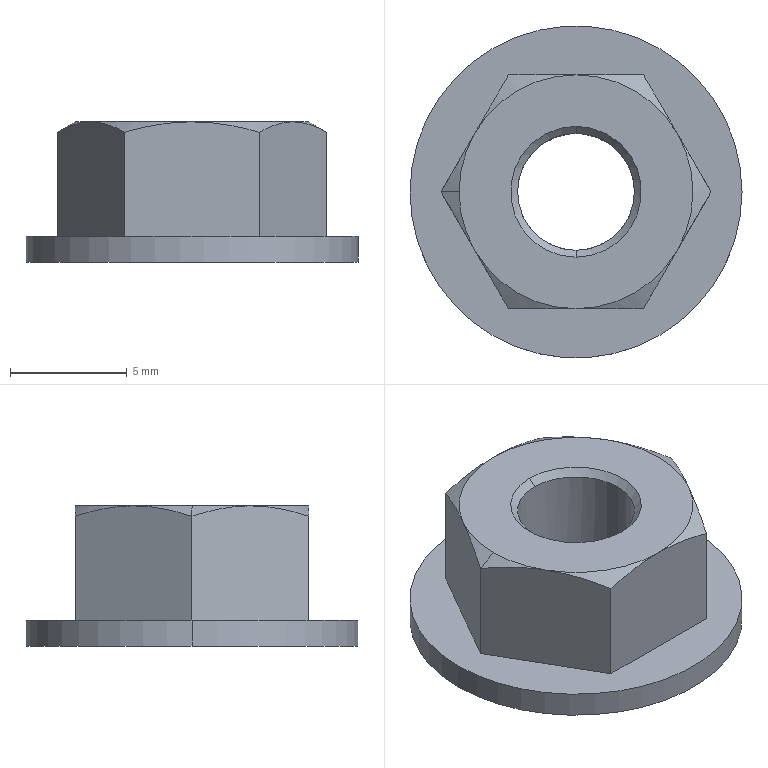Part | STEP file | LE-FL-M6_PN_0003 | 1 solid | 24 faces | box 14.2 x 14.2 x 6 mm | volume 478.178 mm3 | cone 11 | plane 9 | cylinder 4 | commonest cylinder face diameters 5 x2 14.2 x2
STEP:
#1=CARTESIAN_POINT('',(-7.1,0.,1.1));
#2=VERTEX_POINT('',#1);
#3=CARTESIAN_POINT('',(7.1,0.,1.1));
#4=VERTEX_POINT('',#3);
#5=CARTESIAN_POINT('',(0.,0.,1.1));
#6=DIRECTION('',(0.,0.,-1.));
#7=DIRECTION('',(-1.,0.,0.));
#8=AXIS2_PLACEMENT_3D('',#5,#6,#7);
#9=CIRCLE('',#8,7.1);
#10=EDGE_CURVE('',#2,#4,#9,.T.);
#11=ORIENTED_EDGE('',*,*,#10,.T.);
#12=CARTESIAN_POINT('',(7.1,0.,0.));
#13=VERTEX_POINT('',#12);
#14=CARTESIAN_POINT('',(7.1,0.,6.));
#15=DIRECTION('',(0.,0.,-1.));
#16=VECTOR('',#15,1000.);
#17=LINE('',#14,#16);
#18=EDGE_CURVE('',#4,#13,#17,.T.);
#19=ORIENTED_EDGE('',*,*,#18,.T.);
#20=CARTESIAN_POINT('',(-7.1,0.,0.));
#21=VERTEX_POINT('',#20);
#22=CARTESIAN_POINT('',(0.,0.,0.));
#23=DIRECTION('',(0.,0.,1.));
#24=DIRECTION('',(-1.,0.,0.));
#25=AXIS2_PLACEMENT_3D('',#22,#23,#24);
#26=CIRCLE('',#25,7.1);
#27=EDGE_CURVE('',#13,#21,#26,.T.);
#28=ORIENTED_EDGE('',*,*,#27,.T.);
#29=CARTESIAN_POINT('',(-7.1,0.,6.));
#30=DIRECTION('',(0.,0.,-1.));
#31=VECTOR('',#30,1000.);
#32=LINE('',#29,#31);
#33=EDGE_CURVE('',#2,#21,#32,.T.);
#34=ORIENTED_EDGE('',*,*,#33,.F.);
#35=EDGE_LOOP('',(#11,#19,#28,#34));
#36=FACE_OUTER_BOUND('',#35,.T.);
#37=CARTESIAN_POINT('',(0.,0.,6.));
#38=DIRECTION('',(0.,0.,-1.));
#39=DIRECTION('',(-1.,0.,0.));
#40=AXIS2_PLACEMENT_3D('',#37,#38,#39);
#41=CYLINDRICAL_SURFACE('',#40,7.1);
#42=ADVANCED_FACE('',(#36),#41,.T.);
#43=CARTESIAN_POINT('',(2.5,0.,0.3));
#44=VERTEX_POINT('',#43);
#45=CARTESIAN_POINT('',(-2.5,0.,0.3));
#46=VERTEX_POINT('',#45);
#47=CARTESIAN_POINT('',(0.,0.,0.3));
#48=DIRECTION('',(0.,0.,-1.));
#49=DIRECTION('',(-1.,0.,0.));
#50=AXIS2_PLACEMENT_3D('',#47,#48,#49);
#51=CIRCLE('',#50,2.5);
#52=EDGE_CURVE('',#44,#46,#51,.T.);
#53=ORIENTED_EDGE('',*,*,#52,.F.);
#54=CARTESIAN_POINT('',(2.8,0.,0.));
#55=VERTEX_POINT('',#54);
#56=CARTESIAN_POINT('',(2.8,0.,0.));
#57=DIRECTION('',(0.7071,0.,-0.7071));
#58=VECTOR('',#57,1000.);
#59=LINE('',#56,#58);
#60=EDGE_CURVE('',#44,#55,#59,.T.);
#61=ORIENTED_EDGE('',*,*,#60,.T.);
#62=CARTESIAN_POINT('',(-2.8,0.,0.));
#63=VERTEX_POINT('',#62);
#64=CARTESIAN_POINT('',(0.,0.,0.));
#65=DIRECTION('',(0.,0.,-1.));
#66=DIRECTION('',(-1.,0.,0.));
#67=AXIS2_PLACEMENT_3D('',#64,#65,#66);
#68=CIRCLE('',#67,2.8);
#69=EDGE_CURVE('',#55,#63,#68,.T.);
#70=ORIENTED_EDGE('',*,*,#69,.T.);
#71=CARTESIAN_POINT('',(-2.8,0.,0.));
#72=DIRECTION('',(-0.7071,0.,-0.7071));
#73=VECTOR('',#72,1000.);
#74=LINE('',#71,#73);
#75=EDGE_CURVE('',#46,#63,#74,.T.);
#76=ORIENTED_EDGE('',*,*,#75,.F.);
#77=EDGE_LOOP('',(#53,#61,#70,#76));
#78=FACE_OUTER_BOUND('',#77,.T.);
#79=CARTESIAN_POINT('',(0.,0.,0.));
#80=DIRECTION('',(0.,0.,-1.));
#81=DIRECTION('',(-1.,0.,0.));
#82=AXIS2_PLACEMENT_3D('',#79,#80,#81);
#83=CONICAL_SURFACE('',#82,2.8,0.7854);
#84=ADVANCED_FACE('',(#78),#83,.F.);
#85=ORIENTED_EDGE('',*,*,#52,.T.);
#86=CARTESIAN_POINT('',(-2.5,0.,5.7));
#87=VERTEX_POINT('',#86);
#88=CARTESIAN_POINT('',(-2.5,0.,6.));
#89=DIRECTION('',(0.,0.,1.));
#90=VECTOR('',#89,1000.);
#91=LINE('',#88,#90);
#92=EDGE_CURVE('',#46,#87,#91,.T.);
#93=ORIENTED_EDGE('',*,*,#92,.T.);
#94=CARTESIAN_POINT('',(0.,-2.5,5.7));
#95=VERTEX_POINT('',#94);
#96=CARTESIAN_POINT('',(0.,0.,5.7));
#97=DIRECTION('',(0.,0.,-1.));
#98=DIRECTION('',(1.,0.,0.));
#99=AXIS2_PLACEMENT_3D('',#96,#97,#98);
#100=CIRCLE('',#99,2.5);
#101=EDGE_CURVE('',#95,#87,#100,.T.);
#102=ORIENTED_EDGE('',*,*,#101,.F.);
#103=CARTESIAN_POINT('',(2.5,0.,5.7));
#104=VERTEX_POINT('',#103);
#105=CARTESIAN_POINT('',(0.,0.,5.7));
#106=DIRECTION('',(0.,0.,-1.));
#107=DIRECTION('',(1.,0.,0.));
#108=AXIS2_PLACEMENT_3D('',#105,#106,#107);
#109=CIRCLE('',#108,2.5);
#110=EDGE_CURVE('',#104,#95,#109,.T.);
#111=ORIENTED_EDGE('',*,*,#110,.F.);
#112=CARTESIAN_POINT('',(2.5,0.,6.));
#113=DIRECTION('',(0.,0.,1.));
#114=VECTOR('',#113,1000.);
#115=LINE('',#112,#114);
#116=EDGE_CURVE('',#44,#104,#115,.T.);
#117=ORIENTED_EDGE('',*,*,#116,.F.);
#118=EDGE_LOOP('',(#85,#93,#102,#111,#117));
#119=FACE_OUTER_BOUND('',#118,.T.);
#120=CARTESIAN_POINT('',(0.,0.,6.));
#121=DIRECTION('',(0.,0.,1.));
#122=DIRECTION('',(1.,0.,0.));
#123=AXIS2_PLACEMENT_3D('',#120,#121,#122);
#124=CYLINDRICAL_SURFACE('',#123,2.5);
#125=ADVANCED_FACE('',(#119),#124,.F.);
#126=ORIENTED_EDGE('',*,*,#101,.T.);
#127=CARTESIAN_POINT('',(0.,2.5,5.7));
#128=VERTEX_POINT('',#127);
#129=CARTESIAN_POINT('',(0.,0.,5.7));
#130=DIRECTION('',(0.,0.,-1.));
#131=DIRECTION('',(1.,0.,0.));
#132=AXIS2_PLACEMENT_3D('',#129,#130,#131);
#133=CIRCLE('',#132,2.5);
#134=EDGE_CURVE('',#87,#128,#133,.T.);
#135=ORIENTED_EDGE('',*,*,#134,.T.);
#136=CARTESIAN_POINT('',(0.,2.8,6.));
#137=VERTEX_POINT('',#136);
#138=CARTESIAN_POINT('',(0.,2.8,6.));
#139=DIRECTION('',(0.,0.7071,0.7071));
#140=VECTOR('',#139,1000.);
#141=LINE('',#138,#140);
#142=EDGE_CURVE('',#128,#137,#141,.T.);
#143=ORIENTED_EDGE('',*,*,#142,.T.);
#144=CARTESIAN_POINT('',(0.,-2.8,6.));
#145=VERTEX_POINT('',#144);
#146=CARTESIAN_POINT('',(0.,0.,6.));
#147=DIRECTION('',(0.,0.,-1.));
#148=DIRECTION('',(0.,-1.,0.));
#149=AXIS2_PLACEMENT_3D('',#146,#147,#148);
#150=CIRCLE('',#149,2.8);
#151=EDGE_CURVE('',#145,#137,#150,.T.);
#152=ORIENTED_EDGE('',*,*,#151,.F.);
#153=CARTESIAN_POINT('',(0.,-2.8,6.));
#154=DIRECTION('',(0.,-0.7071,0.7071));
#155=VECTOR('',#154,1000.);
#156=LINE('',#153,#155);
#157=EDGE_CURVE('',#95,#145,#156,.T.);
#158=ORIENTED_EDGE('',*,*,#157,.F.);
#159=EDGE_LOOP('',(#126,#135,#143,#152,#158));
#160=FACE_OUTER_BOUND('',#159,.T.);
#161=CARTESIAN_POINT('',(0.,0.,6.));
#162=DIRECTION('',(0.,0.,1.));
#163=DIRECTION('',(0.,-1.,0.));
#164=AXIS2_PLACEMENT_3D('',#161,#162,#163);
#165=CONICAL_SURFACE('',#164,2.8,0.7854);
#166=ADVANCED_FACE('',(#160),#165,.F.);
#167=CARTESIAN_POINT('',(-4.33,-2.5,6.));
#168=VERTEX_POINT('',#167);
#169=CARTESIAN_POINT('',(-5.,0.,6.));
#170=VERTEX_POINT('',#169);
#171=CARTESIAN_POINT('',(0.,0.,6.));
#172=DIRECTION('',(0.,0.,-1.));
#173=DIRECTION('',(-1.,0.,0.));
#174=AXIS2_PLACEMENT_3D('',#171,#172,#173);
#175=CIRCLE('',#174,5.);
#176=EDGE_CURVE('',#168,#170,#175,.T.);
#177=ORIENTED_EDGE('',*,*,#176,.T.);
#178=CARTESIAN_POINT('',(-5.774,0.,5.553));
#179=VERTEX_POINT('',#178);
#180=CARTESIAN_POINT('',(-5.778,0.,5.551));
#181=DIRECTION('',(-0.866,0.,-0.5));
#182=VECTOR('',#181,1000.);
#183=LINE('',#180,#182);
#184=EDGE_CURVE('',#170,#179,#183,.T.);
#185=ORIENTED_EDGE('',*,*,#184,.T.);
#186=CARTESIAN_POINT('',(-4.33,-2.5,6.));
#187=CARTESIAN_POINT('',(-4.823,-1.647,6.));
#188=CARTESIAN_POINT('',(-5.302,-0.8168,5.826));
#189=CARTESIAN_POINT('',(-5.774,0.,5.553));
#190=B_SPLINE_CURVE_WITH_KNOTS('',3,(#186,#187,#188,#189),.UNSPECIFIED.,.F.,.F.,(4,4),(0.,0.002921),.UNSPECIFIED.);
#191=EDGE_CURVE('',#168,#179,#190,.T.);
#192=ORIENTED_EDGE('',*,*,#191,.F.);
#193=EDGE_LOOP('',(#177,#185,#192));
#194=FACE_OUTER_BOUND('',#193,.T.);
#195=CARTESIAN_POINT('',(0.,0.,5.551));
#196=DIRECTION('',(0.,0.,-1.));
#197=DIRECTION('',(-1.,0.,0.));
#198=AXIS2_PLACEMENT_3D('',#195,#196,#197);
#199=CONICAL_SURFACE('',#198,5.778,1.047);
#200=ADVANCED_FACE('',(#194),#199,.T.);
#201=CARTESIAN_POINT('',(0.,0.,0.));
#202=DIRECTION('',(0.,0.,1.));
#203=DIRECTION('',(-1.,0.,0.));
#204=AXIS2_PLACEMENT_3D('',#201,#202,#203);
#205=CIRCLE('',#204,7.1);
#206=EDGE_CURVE('',#21,#13,#205,.T.);
#207=ORIENTED_EDGE('',*,*,#206,.F.);
#208=ORIENTED_EDGE('',*,*,#27,.F.);
#209=EDGE_LOOP('',(#207,#208));
#210=FACE_OUTER_BOUND('',#209,.T.);
#211=CARTESIAN_POINT('',(0.,0.,0.));
#212=DIRECTION('',(0.,0.,-1.));
#213=DIRECTION('',(-1.,0.,0.));
#214=AXIS2_PLACEMENT_3D('',#211,#212,#213);
#215=CIRCLE('',#214,2.8);
#216=EDGE_CURVE('',#63,#55,#215,.T.);
#217=ORIENTED_EDGE('',*,*,#216,.F.);
#218=ORIENTED_EDGE('',*,*,#69,.F.);
#219=EDGE_LOOP('',(#217,#218));
#220=FACE_BOUND('',#219,.T.);
#221=CARTESIAN_POINT('',(0.,0.,0.));
#222=DIRECTION('',(0.,0.,1.));
#223=DIRECTION('',(1.,0.,0.));
#224=AXIS2_PLACEMENT_3D('',#221,#222,#223);
#225=PLANE('',#224);
#226=ADVANCED_FACE('',(#210,#220),#225,.F.);
#227=ORIENTED_EDGE('',*,*,#18,.F.);
#228=CARTESIAN_POINT('',(0.,0.,1.1));
#229=DIRECTION('',(0.,0.,-1.));
#230=DIRECTION('',(-1.,0.,0.));
#231=AXIS2_PLACEMENT_3D('',#228,#229,#230);
#232=CIRCLE('',#231,7.1);
#233=EDGE_CURVE('',#4,#2,#232,.T.);
#234=ORIENTED_EDGE('',*,*,#233,.T.);
#235=ORIENTED_EDGE('',*,*,#33,.T.);
#236=ORIENTED_EDGE('',*,*,#206,.T.);
#237=EDGE_LOOP('',(#227,#234,#235,#236));
#238=FACE_OUTER_BOUND('',#237,.T.);
#239=CARTESIAN_POINT('',(0.,0.,6.));
#240=DIRECTION('',(0.,0.,-1.));
#241=DIRECTION('',(-1.,0.,0.));
#242=AXIS2_PLACEMENT_3D('',#239,#240,#241);
#243=CYLINDRICAL_SURFACE('',#242,7.1);
#244=ADVANCED_FACE('',(#238),#243,.T.);
#245=ORIENTED_EDGE('',*,*,#60,.F.);
#246=CARTESIAN_POINT('',(0.,0.,0.3));
#247=DIRECTION('',(0.,0.,-1.));
#248=DIRECTION('',(-1.,0.,0.));
#249=AXIS2_PLACEMENT_3D('',#246,#247,#248);
#250=CIRCLE('',#249,2.5);
#251=EDGE_CURVE('',#46,#44,#250,.T.);
#252=ORIENTED_EDGE('',*,*,#251,.F.);
#253=ORIENTED_EDGE('',*,*,#75,.T.);
#254=ORIENTED_EDGE('',*,*,#216,.T.);
#255=EDGE_LOOP('',(#245,#252,#253,#254));
#256=FACE_OUTER_BOUND('',#255,.T.);
#257=CARTESIAN_POINT('',(0.,0.,0.));
#258=DIRECTION('',(0.,0.,-1.));
#259=DIRECTION('',(-1.,0.,0.));
#260=AXIS2_PLACEMENT_3D('',#257,#258,#259);
#261=CONICAL_SURFACE('',#260,2.8,0.7854);
#262=ADVANCED_FACE('',(#256),#261,.F.);
#263=ORIENTED_EDGE('',*,*,#10,.F.);
#264=ORIENTED_EDGE('',*,*,#233,.F.);
#265=EDGE_LOOP('',(#263,#264));
#266=FACE_OUTER_BOUND('',#265,.T.);
#267=CARTESIAN_POINT('',(-2.887,5.,1.1));
#268=VERTEX_POINT('',#267);
#269=CARTESIAN_POINT('',(2.887,5.,1.1));
#270=VERTEX_POINT('',#269);
#271=CARTESIAN_POINT('',(0.,5.,1.1));
#272=DIRECTION('',(1.,0.,0.));
#273=VECTOR('',#272,1000.);
#274=LINE('',#271,#273);
#275=EDGE_CURVE('',#268,#270,#274,.T.);
#276=ORIENTED_EDGE('',*,*,#275,.T.);
#277=CARTESIAN_POINT('',(5.774,0.,1.1));
#278=VERTEX_POINT('',#277);
#279=CARTESIAN_POINT('',(2.887,5.,1.1));
#280=DIRECTION('',(0.5,-0.866,0.));
#281=VECTOR('',#280,1000.);
#282=LINE('',#279,#281);
#283=EDGE_CURVE('',#270,#278,#282,.T.);
#284=ORIENTED_EDGE('',*,*,#283,.T.);
#285=CARTESIAN_POINT('',(2.887,-5.,1.1));
#286=VERTEX_POINT('',#285);
#287=CARTESIAN_POINT('',(5.774,0.,1.1));
#288=DIRECTION('',(-0.5,-0.866,0.));
#289=VECTOR('',#288,1000.);
#290=LINE('',#287,#289);
#291=EDGE_CURVE('',#278,#286,#290,.T.);
#292=ORIENTED_EDGE('',*,*,#291,.T.);
#293=CARTESIAN_POINT('',(-2.887,-5.,1.1));
#294=VERTEX_POINT('',#293);
#295=CARTESIAN_POINT('',(0.,-5.,1.1));
#296=DIRECTION('',(-1.,0.,0.));
#297=VECTOR('',#296,1000.);
#298=LINE('',#295,#297);
#299=EDGE_CURVE('',#286,#294,#298,.T.);
#300=ORIENTED_EDGE('',*,*,#299,.T.);
#301=CARTESIAN_POINT('',(-5.774,0.,1.1));
#302=VERTEX_POINT('',#301);
#303=CARTESIAN_POINT('',(-2.887,-5.,1.1));
#304=DIRECTION('',(-0.5,0.866,0.));
#305=VECTOR('',#304,1000.);
#306=LINE('',#303,#305);
#307=EDGE_CURVE('',#294,#302,#306,.T.);
#308=ORIENTED_EDGE('',*,*,#307,.T.);
#309=CARTESIAN_POINT('',(-5.774,0.,1.1));
#310=DIRECTION('',(0.5,0.866,0.));
#311=VECTOR('',#310,1000.);
#312=LINE('',#309,#311);
#313=EDGE_CURVE('',#302,#268,#312,.T.);
#314=ORIENTED_EDGE('',*,*,#313,.T.);
#315=EDGE_LOOP('',(#276,#284,#292,#300,#308,#314));
#316=FACE_BOUND('',#315,.T.);
#317=CARTESIAN_POINT('',(0.,0.,1.1));
#318=DIRECTION('',(0.,0.,1.));
#319=DIRECTION('',(1.,0.,0.));
#320=AXIS2_PLACEMENT_3D('',#317,#318,#319);
#321=PLANE('',#320);
#322=ADVANCED_FACE('',(#266,#316),#321,.T.);
#323=ORIENTED_EDGE('',*,*,#92,.F.);
#324=ORIENTED_EDGE('',*,*,#251,.T.);
#325=ORIENTED_EDGE('',*,*,#116,.T.);
#326=CARTESIAN_POINT('',(0.,0.,5.7));
#327=DIRECTION('',(0.,0.,-1.));
#328=DIRECTION('',(1.,0.,0.));
#329=AXIS2_PLACEMENT_3D('',#326,#327,#328);
#330=CIRCLE('',#329,2.5);
#331=EDGE_CURVE('',#128,#104,#330,.T.);
#332=ORIENTED_EDGE('',*,*,#331,.F.);
#333=ORIENTED_EDGE('',*,*,#134,.F.);
#334=EDGE_LOOP('',(#323,#324,#325,#332,#333));
#335=FACE_OUTER_BOUND('',#334,.T.);
#336=CARTESIAN_POINT('',(0.,0.,6.));
#337=DIRECTION('',(0.,0.,1.));
#338=DIRECTION('',(1.,0.,0.));
#339=AXIS2_PLACEMENT_3D('',#336,#337,#338);
#340=CYLINDRICAL_SURFACE('',#339,2.5);
#341=ADVANCED_FACE('',(#335),#340,.F.);
#342=CARTESIAN_POINT('',(2.887,5.,5.553));
#343=VERTEX_POINT('',#342);
#344=CARTESIAN_POINT('',(4.33,2.5,6.));
#345=VERTEX_POINT('',#344);
#346=CARTESIAN_POINT('',(2.887,5.,5.553));
#347=CARTESIAN_POINT('',(3.358,4.183,5.826));
#348=CARTESIAN_POINT('',(3.837,3.353,6.));
#349=CARTESIAN_POINT('',(4.33,2.5,6.));
#350=B_SPLINE_CURVE_WITH_KNOTS('',3,(#346,#347,#348,#349),.UNSPECIFIED.,.F.,.F.,(4,4),(0.,0.002921),.UNSPECIFIED.);
#351=EDGE_CURVE('',#343,#345,#350,.T.);
#352=ORIENTED_EDGE('',*,*,#351,.T.);
#353=CARTESIAN_POINT('',(5.774,0.,5.553));
#354=VERTEX_POINT('',#353);
#355=CARTESIAN_POINT('',(4.33,2.5,6.));
#356=CARTESIAN_POINT('',(4.823,1.647,6.));
#357=CARTESIAN_POINT('',(5.302,0.8168,5.826));
#358=CARTESIAN_POINT('',(5.774,0.,5.553));
#359=B_SPLINE_CURVE_WITH_KNOTS('',3,(#355,#356,#357,#358),.UNSPECIFIED.,.F.,.F.,(4,4),(0.,0.002921),.UNSPECIFIED.);
#360=EDGE_CURVE('',#345,#354,#359,.T.);
#361=ORIENTED_EDGE('',*,*,#360,.T.);
#362=CARTESIAN_POINT('',(5.774,0.,1.1));
#363=DIRECTION('',(0.,0.,-1.));
#364=VECTOR('',#363,1000.);
#365=LINE('',#362,#364);
#366=EDGE_CURVE('',#354,#278,#365,.T.);
#367=ORIENTED_EDGE('',*,*,#366,.T.);
#368=ORIENTED_EDGE('',*,*,#283,.F.);
#369=CARTESIAN_POINT('',(2.887,5.,1.1));
#370=DIRECTION('',(0.,0.,1.));
#371=VECTOR('',#370,1000.);
#372=LINE('',#369,#371);
#373=EDGE_CURVE('',#270,#343,#372,.T.);
#374=ORIENTED_EDGE('',*,*,#373,.T.);
#375=EDGE_LOOP('',(#352,#361,#367,#368,#374));
#376=FACE_OUTER_BOUND('',#375,.T.);
#377=CARTESIAN_POINT('',(5.774,0.,1.1));
#378=DIRECTION('',(0.866,0.5,0.));
#379=DIRECTION('',(-0.5,0.866,0.));
#380=AXIS2_PLACEMENT_3D('',#377,#378,#379);
#381=PLANE('',#380);
#382=ADVANCED_FACE('',(#376),#381,.T.);
#383=CARTESIAN_POINT('',(-2.887,5.,5.553));
#384=VERTEX_POINT('',#383);
#385=CARTESIAN_POINT('',(0.,5.,6.));
#386=VERTEX_POINT('',#385);
#387=CARTESIAN_POINT('',(-2.887,5.,5.553));
#388=CARTESIAN_POINT('',(-1.944,5.,5.826));
#389=CARTESIAN_POINT('',(-0.9853,5.,6.));
#390=CARTESIAN_POINT('',(0.,5.,6.));
#391=B_SPLINE_CURVE_WITH_KNOTS('',3,(#387,#388,#389,#390),.UNSPECIFIED.,.F.,.F.,(4,4),(0.,0.002921),.UNSPECIFIED.);
#392=EDGE_CURVE('',#384,#386,#391,.T.);
#393=ORIENTED_EDGE('',*,*,#392,.T.);
#394=CARTESIAN_POINT('',(0.,5.,6.));
#395=CARTESIAN_POINT('',(0.9853,5.,6.));
#396=CARTESIAN_POINT('',(1.944,5.,5.826));
#397=CARTESIAN_POINT('',(2.887,5.,5.553));
#398=B_SPLINE_CURVE_WITH_KNOTS('',3,(#394,#395,#396,#397),.UNSPECIFIED.,.F.,.F.,(4,4),(0.,0.002921),.UNSPECIFIED.);
#399=EDGE_CURVE('',#386,#343,#398,.T.);
#400=ORIENTED_EDGE('',*,*,#399,.T.);
#401=ORIENTED_EDGE('',*,*,#373,.F.);
#402=ORIENTED_EDGE('',*,*,#275,.F.);
#403=CARTESIAN_POINT('',(-2.887,5.,1.1));
#404=DIRECTION('',(0.,0.,1.));
#405=VECTOR('',#404,1000.);
#406=LINE('',#403,#405);
#407=EDGE_CURVE('',#268,#384,#406,.T.);
#408=ORIENTED_EDGE('',*,*,#407,.T.);
#409=EDGE_LOOP('',(#393,#400,#401,#402,#408));
#410=FACE_OUTER_BOUND('',#409,.T.);
#411=CARTESIAN_POINT('',(2.887,5.,1.1));
#412=DIRECTION('',(0.,1.,0.));
#413=DIRECTION('',(0.,0.,1.));
#414=AXIS2_PLACEMENT_3D('',#411,#412,#413);
#415=PLANE('',#414);
#416=ADVANCED_FACE('',(#410),#415,.T.);
#417=CARTESIAN_POINT('',(-4.33,2.5,6.));
#418=VERTEX_POINT('',#417);
#419=CARTESIAN_POINT('',(-5.774,0.,5.553));
#420=CARTESIAN_POINT('',(-5.302,0.8168,5.826));
#421=CARTESIAN_POINT('',(-4.823,1.647,6.));
#422=CARTESIAN_POINT('',(-4.33,2.5,6.));
#423=B_SPLINE_CURVE_WITH_KNOTS('',3,(#419,#420,#421,#422),.UNSPECIFIED.,.F.,.F.,(4,4),(0.,0.002921),.UNSPECIFIED.);
#424=EDGE_CURVE('',#179,#418,#423,.T.);
#425=ORIENTED_EDGE('',*,*,#424,.T.);
#426=CARTESIAN_POINT('',(-4.33,2.5,6.));
#427=CARTESIAN_POINT('',(-3.837,3.353,6.));
#428=CARTESIAN_POINT('',(-3.358,4.183,5.826));
#429=CARTESIAN_POINT('',(-2.887,5.,5.553));
#430=B_SPLINE_CURVE_WITH_KNOTS('',3,(#426,#427,#428,#429),.UNSPECIFIED.,.F.,.F.,(4,4),(0.,0.002921),.UNSPECIFIED.);
#431=EDGE_CURVE('',#418,#384,#430,.T.);
#432=ORIENTED_EDGE('',*,*,#431,.T.);
#433=ORIENTED_EDGE('',*,*,#407,.F.);
#434=ORIENTED_EDGE('',*,*,#313,.F.);
#435=CARTESIAN_POINT('',(-5.774,0.,1.1));
#436=DIRECTION('',(0.,0.,1.));
#437=VECTOR('',#436,1000.);
#438=LINE('',#435,#437);
#439=EDGE_CURVE('',#302,#179,#438,.T.);
#440=ORIENTED_EDGE('',*,*,#439,.T.);
#441=EDGE_LOOP('',(#425,#432,#433,#434,#440));
#442=FACE_OUTER_BOUND('',#441,.T.);
#443=CARTESIAN_POINT('',(-2.887,5.,1.1));
#444=DIRECTION('',(-0.866,0.5,0.));
#445=DIRECTION('',(-0.5,-0.866,0.));
#446=AXIS2_PLACEMENT_3D('',#443,#444,#445);
#447=PLANE('',#446);
#448=ADVANCED_FACE('',(#442),#447,.T.);
#449=CARTESIAN_POINT('',(-2.887,-5.,5.553));
#450=VERTEX_POINT('',#449);
#451=CARTESIAN_POINT('',(-2.887,-5.,5.553));
#452=CARTESIAN_POINT('',(-3.358,-4.183,5.826));
#453=CARTESIAN_POINT('',(-3.837,-3.353,6.));
#454=CARTESIAN_POINT('',(-4.33,-2.5,6.));
#455=B_SPLINE_CURVE_WITH_KNOTS('',3,(#451,#452,#453,#454),.UNSPECIFIED.,.F.,.F.,(4,4),(0.,0.002921),.UNSPECIFIED.);
#456=EDGE_CURVE('',#450,#168,#455,.T.);
#457=ORIENTED_EDGE('',*,*,#456,.T.);
#458=ORIENTED_EDGE('',*,*,#191,.T.);
#459=ORIENTED_EDGE('',*,*,#439,.F.);
#460=ORIENTED_EDGE('',*,*,#307,.F.);
#461=CARTESIAN_POINT('',(-2.887,-5.,1.1));
#462=DIRECTION('',(0.,0.,1.));
#463=VECTOR('',#462,1000.);
#464=LINE('',#461,#463);
#465=EDGE_CURVE('',#294,#450,#464,.T.);
#466=ORIENTED_EDGE('',*,*,#465,.T.);
#467=EDGE_LOOP('',(#457,#458,#459,#460,#466));
#468=FACE_OUTER_BOUND('',#467,.T.);
#469=CARTESIAN_POINT('',(-5.774,0.,1.1));
#470=DIRECTION('',(-0.866,-0.5,0.));
#471=DIRECTION('',(0.5,-0.866,0.));
#472=AXIS2_PLACEMENT_3D('',#469,#470,#471);
#473=PLANE('',#472);
#474=ADVANCED_FACE('',(#468),#473,.T.);
#475=CARTESIAN_POINT('',(2.887,-5.,5.553));
#476=VERTEX_POINT('',#475);
#477=CARTESIAN_POINT('',(0.,-5.,6.));
#478=VERTEX_POINT('',#477);
#479=CARTESIAN_POINT('',(2.887,-5.,5.553));
#480=CARTESIAN_POINT('',(1.944,-5.,5.826));
#481=CARTESIAN_POINT('',(0.9853,-5.,6.));
#482=CARTESIAN_POINT('',(0.,-5.,6.));
#483=B_SPLINE_CURVE_WITH_KNOTS('',3,(#479,#480,#481,#482),.UNSPECIFIED.,.F.,.F.,(4,4),(0.,0.002921),.UNSPECIFIED.);
#484=EDGE_CURVE('',#476,#478,#483,.T.);
#485=ORIENTED_EDGE('',*,*,#484,.T.);
#486=CARTESIAN_POINT('',(0.,-5.,6.));
#487=CARTESIAN_POINT('',(-0.9853,-5.,6.));
#488=CARTESIAN_POINT('',(-1.944,-5.,5.826));
#489=CARTESIAN_POINT('',(-2.887,-5.,5.553));
#490=B_SPLINE_CURVE_WITH_KNOTS('',3,(#486,#487,#488,#489),.UNSPECIFIED.,.F.,.F.,(4,4),(0.,0.002921),.UNSPECIFIED.);
#491=EDGE_CURVE('',#478,#450,#490,.T.);
#492=ORIENTED_EDGE('',*,*,#491,.T.);
#493=ORIENTED_EDGE('',*,*,#465,.F.);
#494=ORIENTED_EDGE('',*,*,#299,.F.);
#495=CARTESIAN_POINT('',(2.887,-5.,1.1));
#496=DIRECTION('',(0.,0.,1.));
#497=VECTOR('',#496,1000.);
#498=LINE('',#495,#497);
#499=EDGE_CURVE('',#286,#476,#498,.T.);
#500=ORIENTED_EDGE('',*,*,#499,.T.);
#501=EDGE_LOOP('',(#485,#492,#493,#494,#500));
#502=FACE_OUTER_BOUND('',#501,.T.);
#503=CARTESIAN_POINT('',(-2.887,-5.,1.1));
#504=DIRECTION('',(0.,-1.,0.));
#505=DIRECTION('',(0.,0.,-1.));
#506=AXIS2_PLACEMENT_3D('',#503,#504,#505);
#507=PLANE('',#506);
#508=ADVANCED_FACE('',(#502),#507,.T.);
#509=CARTESIAN_POINT('',(4.33,-2.5,6.));
#510=VERTEX_POINT('',#509);
#511=CARTESIAN_POINT('',(5.774,0.,5.553));
#512=CARTESIAN_POINT('',(5.302,-0.8168,5.826));
#513=CARTESIAN_POINT('',(4.823,-1.647,6.));
#514=CARTESIAN_POINT('',(4.33,-2.5,6.));
#515=B_SPLINE_CURVE_WITH_KNOTS('',3,(#511,#512,#513,#514),.UNSPECIFIED.,.F.,.F.,(4,4),(0.,0.002921),.UNSPECIFIED.);
#516=EDGE_CURVE('',#354,#510,#515,.T.);
#517=ORIENTED_EDGE('',*,*,#516,.T.);
#518=CARTESIAN_POINT('',(4.33,-2.5,6.));
#519=CARTESIAN_POINT('',(3.837,-3.353,6.));
#520=CARTESIAN_POINT('',(3.358,-4.183,5.826));
#521=CARTESIAN_POINT('',(2.887,-5.,5.553));
#522=B_SPLINE_CURVE_WITH_KNOTS('',3,(#518,#519,#520,#521),.UNSPECIFIED.,.F.,.F.,(4,4),(0.,0.002921),.UNSPECIFIED.);
#523=EDGE_CURVE('',#510,#476,#522,.T.);
#524=ORIENTED_EDGE('',*,*,#523,.T.);
#525=ORIENTED_EDGE('',*,*,#499,.F.);
#526=ORIENTED_EDGE('',*,*,#291,.F.);
#527=ORIENTED_EDGE('',*,*,#366,.F.);
#528=EDGE_LOOP('',(#517,#524,#525,#526,#527));
#529=FACE_OUTER_BOUND('',#528,.T.);
#530=CARTESIAN_POINT('',(2.887,-5.,1.1));
#531=DIRECTION('',(0.866,-0.5,0.));
#532=DIRECTION('',(0.5,0.866,0.));
#533=AXIS2_PLACEMENT_3D('',#530,#531,#532);
#534=PLANE('',#533);
#535=ADVANCED_FACE('',(#529),#534,.T.);
#536=ORIENTED_EDGE('',*,*,#142,.F.);
#537=ORIENTED_EDGE('',*,*,#331,.T.);
#538=ORIENTED_EDGE('',*,*,#110,.T.);
#539=ORIENTED_EDGE('',*,*,#157,.T.);
#540=CARTESIAN_POINT('',(0.,0.,6.));
#541=DIRECTION('',(0.,0.,-1.));
#542=DIRECTION('',(0.,-1.,0.));
#543=AXIS2_PLACEMENT_3D('',#540,#541,#542);
#544=CIRCLE('',#543,2.8);
#545=EDGE_CURVE('',#137,#145,#544,.T.);
#546=ORIENTED_EDGE('',*,*,#545,.F.);
#547=EDGE_LOOP('',(#536,#537,#538,#539,#546));
#548=FACE_OUTER_BOUND('',#547,.T.);
#549=CARTESIAN_POINT('',(0.,0.,6.));
#550=DIRECTION('',(0.,0.,1.));
#551=DIRECTION('',(0.,-1.,0.));
#552=AXIS2_PLACEMENT_3D('',#549,#550,#551);
#553=CONICAL_SURFACE('',#552,2.8,0.7854);
#554=ADVANCED_FACE('',(#548),#553,.F.);
#555=ORIENTED_EDGE('',*,*,#516,.F.);
#556=ORIENTED_EDGE('',*,*,#360,.F.);
#557=CARTESIAN_POINT('',(0.,0.,6.));
#558=DIRECTION('',(0.,0.,-1.));
#559=DIRECTION('',(-1.,0.,0.));
#560=AXIS2_PLACEMENT_3D('',#557,#558,#559);
#561=CIRCLE('',#560,5.);
#562=EDGE_CURVE('',#345,#510,#561,.T.);
#563=ORIENTED_EDGE('',*,*,#562,.T.);
#564=EDGE_LOOP('',(#555,#556,#563));
#565=FACE_OUTER_BOUND('',#564,.T.);
#566=CARTESIAN_POINT('',(0.,0.,5.551));
#567=DIRECTION('',(0.,0.,-1.));
#568=DIRECTION('',(-1.,0.,0.));
#569=AXIS2_PLACEMENT_3D('',#566,#567,#568);
#570=CONICAL_SURFACE('',#569,5.778,1.047);
#571=ADVANCED_FACE('',(#565),#570,.T.);
#572=ORIENTED_EDGE('',*,*,#351,.F.);
#573=ORIENTED_EDGE('',*,*,#399,.F.);
#574=CARTESIAN_POINT('',(0.,0.,6.));
#575=DIRECTION('',(0.,0.,-1.));
#576=DIRECTION('',(-1.,0.,0.));
#577=AXIS2_PLACEMENT_3D('',#574,#575,#576);
#578=CIRCLE('',#577,5.);
#579=EDGE_CURVE('',#386,#345,#578,.T.);
#580=ORIENTED_EDGE('',*,*,#579,.T.);
#581=EDGE_LOOP('',(#572,#573,#580));
#582=FACE_OUTER_BOUND('',#581,.T.);
#583=CARTESIAN_POINT('',(0.,0.,5.551));
#584=DIRECTION('',(0.,0.,-1.));
#585=DIRECTION('',(-1.,0.,0.));
#586=AXIS2_PLACEMENT_3D('',#583,#584,#585);
#587=CONICAL_SURFACE('',#586,5.778,1.047);
#588=ADVANCED_FACE('',(#582),#587,.T.);
#589=ORIENTED_EDGE('',*,*,#431,.F.);
#590=CARTESIAN_POINT('',(0.,0.,6.));
#591=DIRECTION('',(0.,0.,-1.));
#592=DIRECTION('',(-1.,0.,0.));
#593=AXIS2_PLACEMENT_3D('',#590,#591,#592);
#594=CIRCLE('',#593,5.);
#595=EDGE_CURVE('',#418,#386,#594,.T.);
#596=ORIENTED_EDGE('',*,*,#595,.T.);
#597=ORIENTED_EDGE('',*,*,#392,.F.);
#598=EDGE_LOOP('',(#589,#596,#597));
#599=FACE_OUTER_BOUND('',#598,.T.);
#600=CARTESIAN_POINT('',(0.,0.,5.551));
#601=DIRECTION('',(0.,0.,-1.));
#602=DIRECTION('',(-1.,0.,0.));
#603=AXIS2_PLACEMENT_3D('',#600,#601,#602);
#604=CONICAL_SURFACE('',#603,5.778,1.047);
#605=ADVANCED_FACE('',(#599),#604,.T.);
#606=ORIENTED_EDGE('',*,*,#184,.F.);
#607=CARTESIAN_POINT('',(0.,0.,6.));
#608=DIRECTION('',(0.,0.,-1.));
#609=DIRECTION('',(-1.,0.,0.));
#610=AXIS2_PLACEMENT_3D('',#607,#608,#609);
#611=CIRCLE('',#610,5.);
#612=EDGE_CURVE('',#170,#418,#611,.T.);
#613=ORIENTED_EDGE('',*,*,#612,.T.);
#614=ORIENTED_EDGE('',*,*,#424,.F.);
#615=EDGE_LOOP('',(#606,#613,#614));
#616=FACE_OUTER_BOUND('',#615,.T.);
#617=CARTESIAN_POINT('',(0.,0.,5.551));
#618=DIRECTION('',(0.,0.,-1.));
#619=DIRECTION('',(-1.,0.,0.));
#620=AXIS2_PLACEMENT_3D('',#617,#618,#619);
#621=CONICAL_SURFACE('',#620,5.778,1.047);
#622=ADVANCED_FACE('',(#616),#621,.T.);
#623=ORIENTED_EDGE('',*,*,#491,.F.);
#624=CARTESIAN_POINT('',(0.,0.,6.));
#625=DIRECTION('',(0.,0.,-1.));
#626=DIRECTION('',(-1.,0.,0.));
#627=AXIS2_PLACEMENT_3D('',#624,#625,#626);
#628=CIRCLE('',#627,5.);
#629=EDGE_CURVE('',#478,#168,#628,.T.);
#630=ORIENTED_EDGE('',*,*,#629,.T.);
#631=ORIENTED_EDGE('',*,*,#456,.F.);
#632=EDGE_LOOP('',(#623,#630,#631));
#633=FACE_OUTER_BOUND('',#632,.T.);
#634=CARTESIAN_POINT('',(0.,0.,5.551));
#635=DIRECTION('',(0.,0.,-1.));
#636=DIRECTION('',(-1.,0.,0.));
#637=AXIS2_PLACEMENT_3D('',#634,#635,#636);
#638=CONICAL_SURFACE('',#637,5.778,1.047);
#639=ADVANCED_FACE('',(#633),#638,.T.);
#640=ORIENTED_EDGE('',*,*,#484,.F.);
#641=ORIENTED_EDGE('',*,*,#523,.F.);
#642=CARTESIAN_POINT('',(0.,0.,6.));
#643=DIRECTION('',(0.,0.,-1.));
#644=DIRECTION('',(-1.,0.,0.));
#645=AXIS2_PLACEMENT_3D('',#642,#643,#644);
#646=CIRCLE('',#645,5.);
#647=EDGE_CURVE('',#510,#478,#646,.T.);
#648=ORIENTED_EDGE('',*,*,#647,.T.);
#649=EDGE_LOOP('',(#640,#641,#648));
#650=FACE_OUTER_BOUND('',#649,.T.);
#651=CARTESIAN_POINT('',(0.,0.,5.551));
#652=DIRECTION('',(0.,0.,-1.));
#653=DIRECTION('',(-1.,0.,0.));
#654=AXIS2_PLACEMENT_3D('',#651,#652,#653);
#655=CONICAL_SURFACE('',#654,5.778,1.047);
#656=ADVANCED_FACE('',(#650),#655,.T.);
#657=ORIENTED_EDGE('',*,*,#647,.F.);
#658=ORIENTED_EDGE('',*,*,#562,.F.);
#659=ORIENTED_EDGE('',*,*,#579,.F.);
#660=ORIENTED_EDGE('',*,*,#595,.F.);
#661=ORIENTED_EDGE('',*,*,#612,.F.);
#662=ORIENTED_EDGE('',*,*,#176,.F.);
#663=ORIENTED_EDGE('',*,*,#629,.F.);
#664=EDGE_LOOP('',(#657,#658,#659,#660,#661,#662,#663));
#665=FACE_OUTER_BOUND('',#664,.T.);
#666=ORIENTED_EDGE('',*,*,#151,.T.);
#667=ORIENTED_EDGE('',*,*,#545,.T.);
#668=EDGE_LOOP('',(#666,#667));
#669=FACE_BOUND('',#668,.T.);
#670=CARTESIAN_POINT('',(0.,0.,6.));
#671=DIRECTION('',(0.,0.,1.));
#672=DIRECTION('',(1.,0.,0.));
#673=AXIS2_PLACEMENT_3D('',#670,#671,#672);
#674=PLANE('',#673);
#675=ADVANCED_FACE('',(#665,#669),#674,.T.);
#676=CLOSED_SHELL('',(#42,#84,#125,#166,#200,#226,#244,#262,#322,#341,#382,#416,#448,#474,#508,#535,#554,#571,#588,#605,#622,#639,#656,#675));
#677=MANIFOLD_SOLID_BREP('',#676);
#678=CARTESIAN_POINT('',(0.,0.,0.));
#679=DIRECTION('',(0.,0.,1.));
#680=DIRECTION('',(1.,0.,0.));
#681=AXIS2_PLACEMENT_3D('',#678,#679,#680);
#682=(LENGTH_UNIT()NAMED_UNIT(*)SI_UNIT(.MILLI.,.METRE.));
#683=UNCERTAINTY_MEASURE_WITH_UNIT(LENGTH_MEASURE(0.00001),#682,'','');
#684=(NAMED_UNIT(*)PLANE_ANGLE_UNIT()SI_UNIT($,.RADIAN.));
#685=(NAMED_UNIT(*)SI_UNIT($,.STERADIAN.)SOLID_ANGLE_UNIT());
#686=(GEOMETRIC_REPRESENTATION_CONTEXT(3)GLOBAL_UNCERTAINTY_ASSIGNED_CONTEXT((#683))GLOBAL_UNIT_ASSIGNED_CONTEXT((#682,#684,#685))REPRESENTATION_CONTEXT('',''));
#687=ADVANCED_BREP_SHAPE_REPRESENTATION('',(#677,#681),#686);